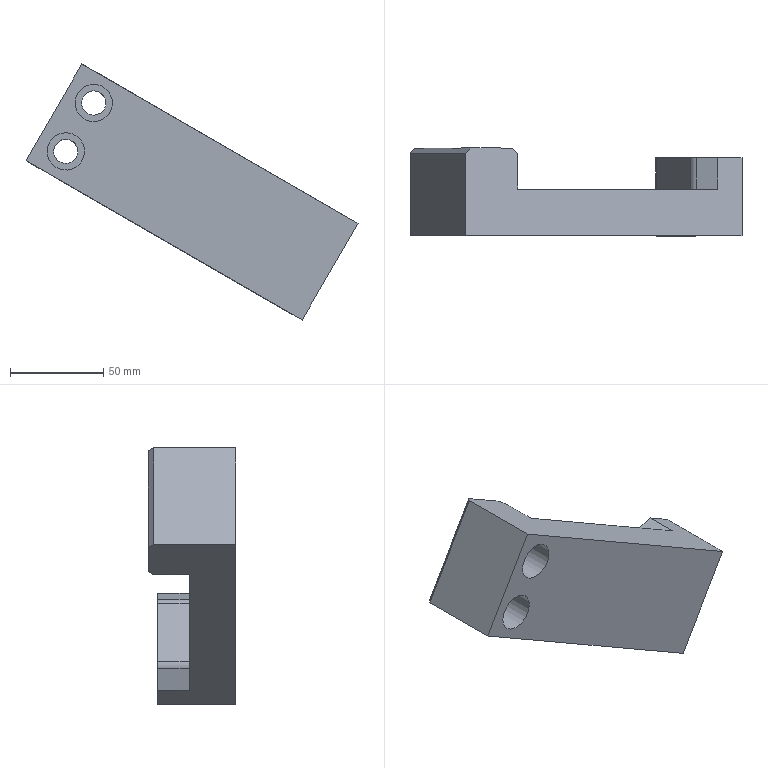Part | NX | features solid 2 | 1 solid | 22 faces | box 178.09 x 47 x 137.462 mm | volume 304062 mm3 | plane 16 | cylinder 6 | commonest cylinder face diameters 10 x2 13 x2 20 x2
STEP:
#1=CARTESIAN_POINT('',(239.,-415.,62.));
#2=VERTEX_POINT('',#1);
#3=CARTESIAN_POINT('',(239.,-371.,62.));
#4=VERTEX_POINT('',#3);
#5=CARTESIAN_POINT('',(239.,-415.,62.));
#6=DIRECTION('',(0.,1.,0.));
#7=VECTOR('',#6,1000.);
#8=LINE('',#5,#7);
#9=EDGE_CURVE('',#2,#4,#8,.T.);
#10=ORIENTED_EDGE('',*,*,#9,.F.);
#11=CARTESIAN_POINT('',(387.09,-415.,-23.5));
#12=VERTEX_POINT('',#11);
#13=CARTESIAN_POINT('',(387.09,-415.,-23.5));
#14=DIRECTION('',(-0.866,0.,0.5));
#15=VECTOR('',#14,1000.);
#16=LINE('',#13,#15);
#17=EDGE_CURVE('',#12,#2,#16,.T.);
#18=ORIENTED_EDGE('',*,*,#17,.F.);
#19=CARTESIAN_POINT('',(387.09,-373.,-23.5));
#20=VERTEX_POINT('',#19);
#21=CARTESIAN_POINT('',(387.09,-415.,-23.5));
#22=DIRECTION('',(0.,1.,0.));
#23=VECTOR('',#22,1000.);
#24=LINE('',#21,#23);
#25=EDGE_CURVE('',#12,#20,#24,.T.);
#26=ORIENTED_EDGE('',*,*,#25,.T.);
#27=CARTESIAN_POINT('',(374.1,-373.,-16.));
#28=VERTEX_POINT('',#27);
#29=CARTESIAN_POINT('',(387.09,-373.,-23.5));
#30=DIRECTION('',(-0.866,0.,0.5));
#31=VECTOR('',#30,1000.);
#32=LINE('',#29,#31);
#33=EDGE_CURVE('',#20,#28,#32,.T.);
#34=ORIENTED_EDGE('',*,*,#33,.T.);
#35=CARTESIAN_POINT('',(374.1,-390.,-16.));
#36=VERTEX_POINT('',#35);
#37=CARTESIAN_POINT('',(374.1,-415.,-16.));
#38=DIRECTION('',(0.,-1.,0.));
#39=VECTOR('',#38,1000.);
#40=LINE('',#37,#39);
#41=EDGE_CURVE('',#36,#28,#40,.F.);
#42=ORIENTED_EDGE('',*,*,#41,.F.);
#43=CARTESIAN_POINT('',(266.713,-390.,46.));
#44=VERTEX_POINT('',#43);
#45=CARTESIAN_POINT('',(387.09,-390.,-23.5));
#46=DIRECTION('',(-0.866,0.,0.5));
#47=VECTOR('',#46,1000.);
#48=LINE('',#45,#47);
#49=EDGE_CURVE('',#36,#44,#48,.T.);
#50=ORIENTED_EDGE('',*,*,#49,.T.);
#51=CARTESIAN_POINT('',(266.713,-371.,46.));
#52=VERTEX_POINT('',#51);
#53=CARTESIAN_POINT('',(266.713,-390.,46.));
#54=DIRECTION('',(0.,1.,0.));
#55=VECTOR('',#54,1000.);
#56=LINE('',#53,#55);
#57=EDGE_CURVE('',#44,#52,#56,.T.);
#58=ORIENTED_EDGE('',*,*,#57,.T.);
#59=CARTESIAN_POINT('',(264.115,-368.,47.5));
#60=VERTEX_POINT('',#59);
#61=CARTESIAN_POINT('',(345.954,-462.5,0.25));
#62=DIRECTION('',(-0.6124,0.7071,0.3536));
#63=VECTOR('',#62,1000.);
#64=LINE('',#61,#63);
#65=EDGE_CURVE('',#60,#52,#64,.F.);
#66=ORIENTED_EDGE('',*,*,#65,.F.);
#67=CARTESIAN_POINT('',(241.598,-368.,60.5));
#68=VERTEX_POINT('',#67);
#69=CARTESIAN_POINT('',(239.,-368.,62.));
#70=DIRECTION('',(0.866,0.,-0.5));
#71=VECTOR('',#70,1000.);
#72=LINE('',#69,#71);
#73=EDGE_CURVE('',#68,#60,#72,.T.);
#74=ORIENTED_EDGE('',*,*,#73,.F.);
#75=CARTESIAN_POINT('',(293.993,-307.5,30.25));
#76=DIRECTION('',(0.6124,0.7071,-0.3536));
#77=VECTOR('',#76,1000.);
#78=LINE('',#75,#77);
#79=EDGE_CURVE('',#4,#68,#78,.T.);
#80=ORIENTED_EDGE('',*,*,#79,.F.);
#81=EDGE_LOOP('',(#10,#18,#26,#34,#42,#50,#58,#66,#74,#80));
#82=FACE_BOUND('',#81,.T.);
#83=CARTESIAN_POINT('',(387.09,-415.,-23.5));
#84=DIRECTION('',(0.5,0.,0.866));
#85=DIRECTION('',(-0.866,0.,0.5));
#86=AXIS2_PLACEMENT_3D('',#83,#84,#85);
#87=PLANE('',#86);
#88=ADVANCED_FACE('',(#82),#87,.T.);
#89=CARTESIAN_POINT('',(359.404,-390.,-21.454));
#90=VERTEX_POINT('',#89);
#91=CARTESIAN_POINT('',(341.475,-390.,-52.508));
#92=VERTEX_POINT('',#91);
#93=CARTESIAN_POINT('',(365.44,-390.,-11.));
#94=DIRECTION('',(-0.5,0.,-0.866));
#95=VECTOR('',#94,1000.);
#96=LINE('',#93,#95);
#97=EDGE_CURVE('',#90,#92,#96,.T.);
#98=ORIENTED_EDGE('',*,*,#97,.F.);
#99=CARTESIAN_POINT('',(359.404,-373.,-21.454));
#100=VERTEX_POINT('',#99);
#101=CARTESIAN_POINT('',(359.404,-390.,-21.454));
#102=DIRECTION('',(0.,1.,0.));
#103=VECTOR('',#102,1000.);
#104=LINE('',#101,#103);
#105=EDGE_CURVE('',#100,#90,#104,.F.);
#106=ORIENTED_EDGE('',*,*,#105,.F.);
#107=CARTESIAN_POINT('',(341.475,-373.,-52.508));
#108=VERTEX_POINT('',#107);
#109=CARTESIAN_POINT('',(365.44,-373.,-11.));
#110=DIRECTION('',(-0.5,0.,-0.866));
#111=VECTOR('',#110,1000.);
#112=LINE('',#109,#111);
#113=EDGE_CURVE('',#100,#108,#112,.T.);
#114=ORIENTED_EDGE('',*,*,#113,.T.);
#115=CARTESIAN_POINT('',(341.475,-390.,-52.508));
#116=DIRECTION('',(0.,-1.,0.));
#117=VECTOR('',#116,1000.);
#118=LINE('',#115,#117);
#119=EDGE_CURVE('',#92,#108,#118,.F.);
#120=ORIENTED_EDGE('',*,*,#119,.F.);
#121=EDGE_LOOP('',(#98,#106,#114,#120));
#122=FACE_BOUND('',#121,.T.);
#123=CARTESIAN_POINT('',(365.44,-390.,-11.));
#124=DIRECTION('',(0.866,0.,-0.5));
#125=DIRECTION('',(-0.5,0.,-0.866));
#126=AXIS2_PLACEMENT_3D('',#123,#124,#125);
#127=PLANE('',#126);
#128=ADVANCED_FACE('',(#122),#127,.F.);
#129=ORIENTED_EDGE('',*,*,#113,.F.);
#130=CARTESIAN_POINT('',(362.44,-373.,-19.124));
#131=VERTEX_POINT('',#130);
#132=CARTESIAN_POINT('',(363.734,-373.,-23.954));
#133=DIRECTION('',(0.,1.,0.));
#134=DIRECTION('',(-0.5,0.,-0.866));
#135=AXIS2_PLACEMENT_3D('',#132,#133,#134);
#136=CIRCLE('',#135,5.);
#137=EDGE_CURVE('',#131,#100,#136,.F.);
#138=ORIENTED_EDGE('',*,*,#137,.F.);
#139=CARTESIAN_POINT('',(360.44,-373.,-19.66));
#140=DIRECTION('',(0.9659,0.,0.2588));
#141=VECTOR('',#140,1000.);
#142=LINE('',#139,#141);
#143=EDGE_CURVE('',#131,#28,#142,.T.);
#144=ORIENTED_EDGE('',*,*,#143,.T.);
#145=ORIENTED_EDGE('',*,*,#33,.F.);
#146=CARTESIAN_POINT('',(357.09,-373.,-75.462));
#147=VERTEX_POINT('',#146);
#148=CARTESIAN_POINT('',(387.09,-373.,-23.5));
#149=DIRECTION('',(-0.5,0.,-0.866));
#150=VECTOR('',#149,1000.);
#151=LINE('',#148,#150);
#152=EDGE_CURVE('',#20,#147,#151,.T.);
#153=ORIENTED_EDGE('',*,*,#152,.T.);
#154=CARTESIAN_POINT('',(344.1,-373.,-67.962));
#155=VERTEX_POINT('',#154);
#156=CARTESIAN_POINT('',(357.09,-373.,-75.462));
#157=DIRECTION('',(-0.866,0.,0.5));
#158=VECTOR('',#157,1000.);
#159=LINE('',#156,#158);
#160=EDGE_CURVE('',#147,#155,#159,.T.);
#161=ORIENTED_EDGE('',*,*,#160,.T.);
#162=CARTESIAN_POINT('',(340.976,-373.,-56.302));
#163=VERTEX_POINT('',#162);
#164=CARTESIAN_POINT('',(340.44,-373.,-54.301));
#165=DIRECTION('',(0.2588,0.,-0.9659));
#166=VECTOR('',#165,1000.);
#167=LINE('',#164,#166);
#168=EDGE_CURVE('',#163,#155,#167,.T.);
#169=ORIENTED_EDGE('',*,*,#168,.F.);
#170=CARTESIAN_POINT('',(345.805,-373.,-55.008));
#171=DIRECTION('',(0.,1.,0.));
#172=DIRECTION('',(-0.5,0.,-0.866));
#173=AXIS2_PLACEMENT_3D('',#170,#171,#172);
#174=CIRCLE('',#173,5.);
#175=EDGE_CURVE('',#108,#163,#174,.F.);
#176=ORIENTED_EDGE('',*,*,#175,.F.);
#177=EDGE_LOOP('',(#129,#138,#144,#145,#153,#161,#169,#176));
#178=FACE_BOUND('',#177,.T.);
#179=CARTESIAN_POINT('',(387.09,-373.,-23.5));
#180=DIRECTION('',(0.,-1.,0.));
#181=DIRECTION('',(-0.5,0.,-0.866));
#182=AXIS2_PLACEMENT_3D('',#179,#180,#181);
#183=PLANE('',#182);
#184=ADVANCED_FACE('',(#178),#183,.F.);
#185=ORIENTED_EDGE('',*,*,#49,.F.);
#186=CARTESIAN_POINT('',(362.44,-390.,-19.124));
#187=VERTEX_POINT('',#186);
#188=CARTESIAN_POINT('',(360.44,-390.,-19.66));
#189=DIRECTION('',(0.9659,0.,0.2588));
#190=VECTOR('',#189,1000.);
#191=LINE('',#188,#190);
#192=EDGE_CURVE('',#187,#36,#191,.T.);
#193=ORIENTED_EDGE('',*,*,#192,.F.);
#194=CARTESIAN_POINT('',(363.734,-390.,-23.954));
#195=DIRECTION('',(0.,1.,0.));
#196=DIRECTION('',(-0.866,0.,0.5));
#197=AXIS2_PLACEMENT_3D('',#194,#195,#196);
#198=CIRCLE('',#197,5.);
#199=EDGE_CURVE('',#90,#187,#198,.T.);
#200=ORIENTED_EDGE('',*,*,#199,.F.);
#201=ORIENTED_EDGE('',*,*,#97,.T.);
#202=CARTESIAN_POINT('',(340.976,-390.,-56.302));
#203=VERTEX_POINT('',#202);
#204=CARTESIAN_POINT('',(345.805,-390.,-55.008));
#205=DIRECTION('',(0.,1.,0.));
#206=DIRECTION('',(-0.866,0.,0.5));
#207=AXIS2_PLACEMENT_3D('',#204,#205,#206);
#208=CIRCLE('',#207,5.);
#209=EDGE_CURVE('',#203,#92,#208,.T.);
#210=ORIENTED_EDGE('',*,*,#209,.F.);
#211=CARTESIAN_POINT('',(344.1,-390.,-67.962));
#212=VERTEX_POINT('',#211);
#213=CARTESIAN_POINT('',(340.44,-390.,-54.301));
#214=DIRECTION('',(0.2588,0.,-0.9659));
#215=VECTOR('',#214,1000.);
#216=LINE('',#213,#215);
#217=EDGE_CURVE('',#203,#212,#216,.T.);
#218=ORIENTED_EDGE('',*,*,#217,.T.);
#219=CARTESIAN_POINT('',(236.713,-390.,-5.962));
#220=VERTEX_POINT('',#219);
#221=CARTESIAN_POINT('',(357.09,-390.,-75.462));
#222=DIRECTION('',(-0.866,0.,0.5));
#223=VECTOR('',#222,1000.);
#224=LINE('',#221,#223);
#225=EDGE_CURVE('',#212,#220,#224,.T.);
#226=ORIENTED_EDGE('',*,*,#225,.T.);
#227=CARTESIAN_POINT('',(266.713,-390.,46.));
#228=DIRECTION('',(-0.5,0.,-0.866));
#229=VECTOR('',#228,1000.);
#230=LINE('',#227,#229);
#231=EDGE_CURVE('',#44,#220,#230,.T.);
#232=ORIENTED_EDGE('',*,*,#231,.F.);
#233=EDGE_LOOP('',(#185,#193,#200,#201,#210,#218,#226,#232));
#234=FACE_BOUND('',#233,.T.);
#235=CARTESIAN_POINT('',(387.09,-390.,-23.5));
#236=DIRECTION('',(0.,-1.,0.));
#237=DIRECTION('',(-0.866,0.,0.5));
#238=AXIS2_PLACEMENT_3D('',#235,#236,#237);
#239=PLANE('',#238);
#240=ADVANCED_FACE('',(#234),#239,.F.);
#241=CARTESIAN_POINT('',(254.017,-415.,36.01));
#242=VERTEX_POINT('',#241);
#243=CARTESIAN_POINT('',(245.356,-415.,41.01));
#244=DIRECTION('',(0.,-1.,0.));
#245=DIRECTION('',(0.866,0.,-0.5));
#246=AXIS2_PLACEMENT_3D('',#243,#244,#245);
#247=CIRCLE('',#246,10.);
#248=EDGE_CURVE('',#242,#242,#247,.T.);
#249=ORIENTED_EDGE('',*,*,#248,.F.);
#250=EDGE_LOOP('',(#249));
#251=FACE_BOUND('',#250,.T.);
#252=CARTESIAN_POINT('',(239.017,-415.,10.029));
#253=VERTEX_POINT('',#252);
#254=CARTESIAN_POINT('',(230.356,-415.,15.029));
#255=DIRECTION('',(0.,-1.,0.));
#256=DIRECTION('',(0.866,0.,-0.5));
#257=AXIS2_PLACEMENT_3D('',#254,#255,#256);
#258=CIRCLE('',#257,10.);
#259=EDGE_CURVE('',#253,#253,#258,.T.);
#260=ORIENTED_EDGE('',*,*,#259,.F.);
#261=EDGE_LOOP('',(#260));
#262=FACE_BOUND('',#261,.T.);
#263=CARTESIAN_POINT('',(357.09,-415.,-75.462));
#264=VERTEX_POINT('',#263);
#265=CARTESIAN_POINT('',(387.09,-415.,-23.5));
#266=DIRECTION('',(0.5,0.,0.866));
#267=VECTOR('',#266,1000.);
#268=LINE('',#265,#267);
#269=EDGE_CURVE('',#12,#264,#268,.F.);
#270=ORIENTED_EDGE('',*,*,#269,.F.);
#271=ORIENTED_EDGE('',*,*,#17,.T.);
#272=CARTESIAN_POINT('',(209.,-415.,10.038));
#273=VERTEX_POINT('',#272);
#274=CARTESIAN_POINT('',(239.,-415.,62.));
#275=DIRECTION('',(0.5,0.,0.866));
#276=VECTOR('',#275,1000.);
#277=LINE('',#274,#276);
#278=EDGE_CURVE('',#2,#273,#277,.F.);
#279=ORIENTED_EDGE('',*,*,#278,.T.);
#280=CARTESIAN_POINT('',(357.09,-415.,-75.462));
#281=DIRECTION('',(-0.866,0.,0.5));
#282=VECTOR('',#281,1000.);
#283=LINE('',#280,#282);
#284=EDGE_CURVE('',#264,#273,#283,.T.);
#285=ORIENTED_EDGE('',*,*,#284,.F.);
#286=EDGE_LOOP('',(#270,#271,#279,#285));
#287=FACE_BOUND('',#286,.T.);
#288=CARTESIAN_POINT('',(387.09,-415.,-23.5));
#289=DIRECTION('',(0.,-1.,0.));
#290=DIRECTION('',(-0.866,0.,0.5));
#291=AXIS2_PLACEMENT_3D('',#288,#289,#290);
#292=PLANE('',#291);
#293=ADVANCED_FACE('',(#251,#262,#287),#292,.T.);
#294=CARTESIAN_POINT('',(209.,-371.,10.038));
#295=VERTEX_POINT('',#294);
#296=CARTESIAN_POINT('',(209.,-415.,10.038));
#297=DIRECTION('',(0.,1.,0.));
#298=VECTOR('',#297,1000.);
#299=LINE('',#296,#298);
#300=EDGE_CURVE('',#273,#295,#299,.T.);
#301=ORIENTED_EDGE('',*,*,#300,.F.);
#302=ORIENTED_EDGE('',*,*,#278,.F.);
#303=ORIENTED_EDGE('',*,*,#9,.T.);
#304=CARTESIAN_POINT('',(239.,-371.,62.));
#305=DIRECTION('',(-0.5,0.,-0.866));
#306=VECTOR('',#305,1000.);
#307=LINE('',#304,#306);
#308=EDGE_CURVE('',#295,#4,#307,.F.);
#309=ORIENTED_EDGE('',*,*,#308,.F.);
#310=EDGE_LOOP('',(#301,#302,#303,#309));
#311=FACE_BOUND('',#310,.T.);
#312=CARTESIAN_POINT('',(239.,-415.,62.));
#313=DIRECTION('',(-0.866,0.,0.5));
#314=DIRECTION('',(0.,1.,0.));
#315=AXIS2_PLACEMENT_3D('',#312,#313,#314);
#316=PLANE('',#315);
#317=ADVANCED_FACE('',(#311),#316,.T.);
#318=ORIENTED_EDGE('',*,*,#25,.F.);
#319=ORIENTED_EDGE('',*,*,#269,.T.);
#320=CARTESIAN_POINT('',(357.09,-415.,-75.462));
#321=DIRECTION('',(0.,1.,0.));
#322=VECTOR('',#321,1000.);
#323=LINE('',#320,#322);
#324=EDGE_CURVE('',#264,#147,#323,.T.);
#325=ORIENTED_EDGE('',*,*,#324,.T.);
#326=ORIENTED_EDGE('',*,*,#152,.F.);
#327=EDGE_LOOP('',(#318,#319,#325,#326));
#328=FACE_BOUND('',#327,.T.);
#329=CARTESIAN_POINT('',(387.09,-415.,-23.5));
#330=DIRECTION('',(-0.866,0.,0.5));
#331=DIRECTION('',(0.,1.,0.));
#332=AXIS2_PLACEMENT_3D('',#329,#330,#331);
#333=PLANE('',#332);
#334=ADVANCED_FACE('',(#328),#333,.F.);
#335=CARTESIAN_POINT('',(211.598,-368.,8.538));
#336=VERTEX_POINT('',#335);
#337=CARTESIAN_POINT('',(234.115,-368.,-4.462));
#338=VERTEX_POINT('',#337);
#339=CARTESIAN_POINT('',(357.09,-368.,-75.462));
#340=DIRECTION('',(-0.866,0.,0.5));
#341=VECTOR('',#340,1000.);
#342=LINE('',#339,#341);
#343=EDGE_CURVE('',#336,#338,#342,.F.);
#344=ORIENTED_EDGE('',*,*,#343,.T.);
#345=CARTESIAN_POINT('',(236.713,-371.,-5.962));
#346=VERTEX_POINT('',#345);
#347=CARTESIAN_POINT('',(236.713,-371.,-5.962));
#348=DIRECTION('',(0.6124,-0.7071,-0.3536));
#349=VECTOR('',#348,1000.);
#350=LINE('',#347,#349);
#351=EDGE_CURVE('',#346,#338,#350,.F.);
#352=ORIENTED_EDGE('',*,*,#351,.F.);
#353=CARTESIAN_POINT('',(236.713,-390.,-5.962));
#354=DIRECTION('',(0.,1.,0.));
#355=VECTOR('',#354,1000.);
#356=LINE('',#353,#355);
#357=EDGE_CURVE('',#220,#346,#356,.T.);
#358=ORIENTED_EDGE('',*,*,#357,.F.);
#359=ORIENTED_EDGE('',*,*,#225,.F.);
#360=CARTESIAN_POINT('',(344.1,-415.,-67.962));
#361=DIRECTION('',(0.,-1.,0.));
#362=VECTOR('',#361,1000.);
#363=LINE('',#360,#362);
#364=EDGE_CURVE('',#155,#212,#363,.T.);
#365=ORIENTED_EDGE('',*,*,#364,.F.);
#366=ORIENTED_EDGE('',*,*,#160,.F.);
#367=ORIENTED_EDGE('',*,*,#324,.F.);
#368=ORIENTED_EDGE('',*,*,#284,.T.);
#369=ORIENTED_EDGE('',*,*,#300,.T.);
#370=CARTESIAN_POINT('',(211.598,-368.,8.538));
#371=DIRECTION('',(-0.6124,-0.7071,0.3536));
#372=VECTOR('',#371,1000.);
#373=LINE('',#370,#372);
#374=EDGE_CURVE('',#336,#295,#373,.T.);
#375=ORIENTED_EDGE('',*,*,#374,.F.);
#376=EDGE_LOOP('',(#344,#352,#358,#359,#365,#366,#367,#368,#369,#375));
#377=FACE_BOUND('',#376,.T.);
#378=CARTESIAN_POINT('',(357.09,-415.,-75.462));
#379=DIRECTION('',(0.5,0.,0.866));
#380=DIRECTION('',(-0.866,0.,0.5));
#381=AXIS2_PLACEMENT_3D('',#378,#379,#380);
#382=PLANE('',#381);
#383=ADVANCED_FACE('',(#377),#382,.F.);
#384=ORIENTED_EDGE('',*,*,#57,.F.);
#385=ORIENTED_EDGE('',*,*,#231,.T.);
#386=ORIENTED_EDGE('',*,*,#357,.T.);
#387=CARTESIAN_POINT('',(266.713,-371.,46.));
#388=DIRECTION('',(0.5,0.,0.866));
#389=VECTOR('',#388,1000.);
#390=LINE('',#387,#389);
#391=EDGE_CURVE('',#52,#346,#390,.F.);
#392=ORIENTED_EDGE('',*,*,#391,.F.);
#393=EDGE_LOOP('',(#384,#385,#386,#392));
#394=FACE_BOUND('',#393,.T.);
#395=CARTESIAN_POINT('',(266.713,-390.,46.));
#396=DIRECTION('',(-0.866,0.,0.5));
#397=DIRECTION('',(-0.5,0.,-0.866));
#398=AXIS2_PLACEMENT_3D('',#395,#396,#397);
#399=PLANE('',#398);
#400=ADVANCED_FACE('',(#394),#399,.F.);
#401=CARTESIAN_POINT('',(242.106,-368.,35.38));
#402=VERTEX_POINT('',#401);
#403=CARTESIAN_POINT('',(245.356,-368.,41.01));
#404=DIRECTION('',(0.,1.,0.));
#405=DIRECTION('',(-0.5,0.,-0.866));
#406=AXIS2_PLACEMENT_3D('',#403,#404,#405);
#407=CIRCLE('',#406,6.5);
#408=EDGE_CURVE('',#402,#402,#407,.F.);
#409=ORIENTED_EDGE('',*,*,#408,.T.);
#410=EDGE_LOOP('',(#409));
#411=FACE_BOUND('',#410,.T.);
#412=CARTESIAN_POINT('',(227.106,-368.,9.4));
#413=VERTEX_POINT('',#412);
#414=CARTESIAN_POINT('',(230.356,-368.,15.029));
#415=DIRECTION('',(0.,1.,0.));
#416=DIRECTION('',(-0.5,0.,-0.866));
#417=AXIS2_PLACEMENT_3D('',#414,#415,#416);
#418=CIRCLE('',#417,6.5);
#419=EDGE_CURVE('',#413,#413,#418,.F.);
#420=ORIENTED_EDGE('',*,*,#419,.T.);
#421=EDGE_LOOP('',(#420));
#422=FACE_BOUND('',#421,.T.);
#423=ORIENTED_EDGE('',*,*,#73,.T.);
#424=CARTESIAN_POINT('',(264.115,-368.,47.5));
#425=DIRECTION('',(-0.5,0.,-0.866));
#426=VECTOR('',#425,1000.);
#427=LINE('',#424,#426);
#428=EDGE_CURVE('',#338,#60,#427,.F.);
#429=ORIENTED_EDGE('',*,*,#428,.F.);
#430=ORIENTED_EDGE('',*,*,#343,.F.);
#431=CARTESIAN_POINT('',(211.598,-368.,8.538));
#432=DIRECTION('',(0.5,0.,0.866));
#433=VECTOR('',#432,1000.);
#434=LINE('',#431,#433);
#435=EDGE_CURVE('',#68,#336,#434,.F.);
#436=ORIENTED_EDGE('',*,*,#435,.F.);
#437=EDGE_LOOP('',(#423,#429,#430,#436));
#438=FACE_BOUND('',#437,.T.);
#439=CARTESIAN_POINT('',(387.09,-368.,-23.5));
#440=DIRECTION('',(0.,-1.,0.));
#441=DIRECTION('',(-0.5,0.,-0.866));
#442=AXIS2_PLACEMENT_3D('',#439,#440,#441);
#443=PLANE('',#442);
#444=ADVANCED_FACE('',(#411,#422,#438),#443,.F.);
#445=ORIENTED_EDGE('',*,*,#168,.T.);
#446=ORIENTED_EDGE('',*,*,#364,.T.);
#447=ORIENTED_EDGE('',*,*,#217,.F.);
#448=CARTESIAN_POINT('',(340.976,-373.,-56.302));
#449=DIRECTION('',(0.,-1.,0.));
#450=VECTOR('',#449,1000.);
#451=LINE('',#448,#450);
#452=EDGE_CURVE('',#163,#203,#451,.T.);
#453=ORIENTED_EDGE('',*,*,#452,.F.);
#454=EDGE_LOOP('',(#445,#446,#447,#453));
#455=FACE_BOUND('',#454,.T.);
#456=CARTESIAN_POINT('',(340.44,-373.,-54.301));
#457=DIRECTION('',(0.9659,0.,0.2588));
#458=DIRECTION('',(0.2588,0.,-0.9659));
#459=AXIS2_PLACEMENT_3D('',#456,#457,#458);
#460=PLANE('',#459);
#461=ADVANCED_FACE('',(#455),#460,.F.);
#462=ORIENTED_EDGE('',*,*,#192,.T.);
#463=ORIENTED_EDGE('',*,*,#41,.T.);
#464=ORIENTED_EDGE('',*,*,#143,.F.);
#465=CARTESIAN_POINT('',(362.44,-373.,-19.124));
#466=DIRECTION('',(0.,-1.,0.));
#467=VECTOR('',#466,1000.);
#468=LINE('',#465,#467);
#469=EDGE_CURVE('',#187,#131,#468,.F.);
#470=ORIENTED_EDGE('',*,*,#469,.F.);
#471=EDGE_LOOP('',(#462,#463,#464,#470));
#472=FACE_BOUND('',#471,.T.);
#473=CARTESIAN_POINT('',(360.44,-373.,-19.66));
#474=DIRECTION('',(0.2588,0.,-0.9659));
#475=DIRECTION('',(0.9659,0.,0.2588));
#476=AXIS2_PLACEMENT_3D('',#473,#474,#475);
#477=PLANE('',#476);
#478=ADVANCED_FACE('',(#472),#477,.F.);
#479=ORIENTED_EDGE('',*,*,#175,.T.);
#480=ORIENTED_EDGE('',*,*,#452,.T.);
#481=ORIENTED_EDGE('',*,*,#209,.T.);
#482=ORIENTED_EDGE('',*,*,#119,.T.);
#483=EDGE_LOOP('',(#479,#480,#481,#482));
#484=FACE_BOUND('',#483,.T.);
#485=CARTESIAN_POINT('',(345.805,-373.,-55.008));
#486=DIRECTION('',(0.,-1.,0.));
#487=DIRECTION('',(-0.5,0.,-0.866));
#488=AXIS2_PLACEMENT_3D('',#485,#486,#487);
#489=CYLINDRICAL_SURFACE('',#488,5.);
#490=ADVANCED_FACE('',(#484),#489,.T.);
#491=ORIENTED_EDGE('',*,*,#137,.T.);
#492=ORIENTED_EDGE('',*,*,#105,.T.);
#493=ORIENTED_EDGE('',*,*,#199,.T.);
#494=ORIENTED_EDGE('',*,*,#469,.T.);
#495=EDGE_LOOP('',(#491,#492,#493,#494));
#496=FACE_BOUND('',#495,.T.);
#497=CARTESIAN_POINT('',(363.734,-390.,-23.954));
#498=DIRECTION('',(0.,-1.,0.));
#499=DIRECTION('',(-0.5,0.,-0.866));
#500=AXIS2_PLACEMENT_3D('',#497,#498,#499);
#501=CYLINDRICAL_SURFACE('',#500,5.);
#502=ADVANCED_FACE('',(#496),#501,.T.);
#503=ORIENTED_EDGE('',*,*,#419,.F.);
#504=EDGE_LOOP('',(#503));
#505=FACE_BOUND('',#504,.T.);
#506=CARTESIAN_POINT('',(235.986,-400.,11.779));
#507=VERTEX_POINT('',#506);
#508=CARTESIAN_POINT('',(230.356,-400.,15.029));
#509=DIRECTION('',(0.,-1.,0.));
#510=DIRECTION('',(0.866,0.,-0.5));
#511=AXIS2_PLACEMENT_3D('',#508,#509,#510);
#512=CIRCLE('',#511,6.5);
#513=EDGE_CURVE('',#507,#507,#512,.T.);
#514=ORIENTED_EDGE('',*,*,#513,.T.);
#515=EDGE_LOOP('',(#514));
#516=FACE_BOUND('',#515,.T.);
#517=CARTESIAN_POINT('',(230.356,-315.,15.029));
#518=DIRECTION('',(0.,1.,0.));
#519=DIRECTION('',(0.866,0.,-0.5));
#520=AXIS2_PLACEMENT_3D('',#517,#518,#519);
#521=CYLINDRICAL_SURFACE('',#520,6.5);
#522=ADVANCED_FACE('',(#505,#516),#521,.F.);
#523=ORIENTED_EDGE('',*,*,#513,.F.);
#524=EDGE_LOOP('',(#523));
#525=FACE_BOUND('',#524,.T.);
#526=CARTESIAN_POINT('',(239.017,-400.,10.029));
#527=VERTEX_POINT('',#526);
#528=CARTESIAN_POINT('',(230.356,-400.,15.029));
#529=DIRECTION('',(0.,-1.,0.));
#530=DIRECTION('',(0.866,0.,-0.5));
#531=AXIS2_PLACEMENT_3D('',#528,#529,#530);
#532=CIRCLE('',#531,10.);
#533=EDGE_CURVE('',#527,#527,#532,.T.);
#534=ORIENTED_EDGE('',*,*,#533,.T.);
#535=EDGE_LOOP('',(#534));
#536=FACE_BOUND('',#535,.T.);
#537=CARTESIAN_POINT('',(230.356,-400.,15.029));
#538=DIRECTION('',(0.,1.,0.));
#539=DIRECTION('',(0.866,0.,-0.5));
#540=AXIS2_PLACEMENT_3D('',#537,#538,#539);
#541=PLANE('',#540);
#542=ADVANCED_FACE('',(#525,#536),#541,.F.);
#543=ORIENTED_EDGE('',*,*,#533,.F.);
#544=EDGE_LOOP('',(#543));
#545=FACE_BOUND('',#544,.T.);
#546=ORIENTED_EDGE('',*,*,#259,.T.);
#547=EDGE_LOOP('',(#546));
#548=FACE_BOUND('',#547,.T.);
#549=CARTESIAN_POINT('',(230.356,-415.,15.029));
#550=DIRECTION('',(0.,1.,0.));
#551=DIRECTION('',(0.866,0.,-0.5));
#552=AXIS2_PLACEMENT_3D('',#549,#550,#551);
#553=CYLINDRICAL_SURFACE('',#552,10.);
#554=ADVANCED_FACE('',(#545,#548),#553,.F.);
#555=ORIENTED_EDGE('',*,*,#408,.F.);
#556=EDGE_LOOP('',(#555));
#557=FACE_BOUND('',#556,.T.);
#558=CARTESIAN_POINT('',(250.986,-400.,37.76));
#559=VERTEX_POINT('',#558);
#560=CARTESIAN_POINT('',(245.356,-400.,41.01));
#561=DIRECTION('',(0.,-1.,0.));
#562=DIRECTION('',(0.866,0.,-0.5));
#563=AXIS2_PLACEMENT_3D('',#560,#561,#562);
#564=CIRCLE('',#563,6.5);
#565=EDGE_CURVE('',#559,#559,#564,.T.);
#566=ORIENTED_EDGE('',*,*,#565,.T.);
#567=EDGE_LOOP('',(#566));
#568=FACE_BOUND('',#567,.T.);
#569=CARTESIAN_POINT('',(245.356,-315.,41.01));
#570=DIRECTION('',(0.,1.,0.));
#571=DIRECTION('',(0.866,0.,-0.5));
#572=AXIS2_PLACEMENT_3D('',#569,#570,#571);
#573=CYLINDRICAL_SURFACE('',#572,6.5);
#574=ADVANCED_FACE('',(#557,#568),#573,.F.);
#575=ORIENTED_EDGE('',*,*,#565,.F.);
#576=EDGE_LOOP('',(#575));
#577=FACE_BOUND('',#576,.T.);
#578=CARTESIAN_POINT('',(254.017,-400.,36.01));
#579=VERTEX_POINT('',#578);
#580=CARTESIAN_POINT('',(245.356,-400.,41.01));
#581=DIRECTION('',(0.,-1.,0.));
#582=DIRECTION('',(0.866,0.,-0.5));
#583=AXIS2_PLACEMENT_3D('',#580,#581,#582);
#584=CIRCLE('',#583,10.);
#585=EDGE_CURVE('',#579,#579,#584,.T.);
#586=ORIENTED_EDGE('',*,*,#585,.T.);
#587=EDGE_LOOP('',(#586));
#588=FACE_BOUND('',#587,.T.);
#589=CARTESIAN_POINT('',(245.356,-400.,41.01));
#590=DIRECTION('',(0.,1.,0.));
#591=DIRECTION('',(0.866,0.,-0.5));
#592=AXIS2_PLACEMENT_3D('',#589,#590,#591);
#593=PLANE('',#592);
#594=ADVANCED_FACE('',(#577,#588),#593,.F.);
#595=ORIENTED_EDGE('',*,*,#585,.F.);
#596=EDGE_LOOP('',(#595));
#597=FACE_BOUND('',#596,.T.);
#598=ORIENTED_EDGE('',*,*,#248,.T.);
#599=EDGE_LOOP('',(#598));
#600=FACE_BOUND('',#599,.T.);
#601=CARTESIAN_POINT('',(245.356,-415.,41.01));
#602=DIRECTION('',(0.,1.,0.));
#603=DIRECTION('',(0.866,0.,-0.5));
#604=AXIS2_PLACEMENT_3D('',#601,#602,#603);
#605=CYLINDRICAL_SURFACE('',#604,10.);
#606=ADVANCED_FACE('',(#597,#600),#605,.F.);
#607=ORIENTED_EDGE('',*,*,#79,.T.);
#608=ORIENTED_EDGE('',*,*,#435,.T.);
#609=ORIENTED_EDGE('',*,*,#374,.T.);
#610=ORIENTED_EDGE('',*,*,#308,.T.);
#611=EDGE_LOOP('',(#607,#608,#609,#610));
#612=FACE_BOUND('',#611,.T.);
#613=CARTESIAN_POINT('',(241.598,-368.,60.5));
#614=DIRECTION('',(-0.6124,0.7071,0.3536));
#615=DIRECTION('',(0.6124,0.7071,-0.3536));
#616=AXIS2_PLACEMENT_3D('',#613,#614,#615);
#617=PLANE('',#616);
#618=ADVANCED_FACE('',(#612),#617,.T.);
#619=ORIENTED_EDGE('',*,*,#65,.T.);
#620=ORIENTED_EDGE('',*,*,#391,.T.);
#621=ORIENTED_EDGE('',*,*,#351,.T.);
#622=ORIENTED_EDGE('',*,*,#428,.T.);
#623=EDGE_LOOP('',(#619,#620,#621,#622));
#624=FACE_BOUND('',#623,.T.);
#625=CARTESIAN_POINT('',(266.713,-371.,46.));
#626=DIRECTION('',(-0.6124,-0.7071,0.3536));
#627=DIRECTION('',(-0.6124,0.7071,0.3536));
#628=AXIS2_PLACEMENT_3D('',#625,#626,#627);
#629=PLANE('',#628);
#630=ADVANCED_FACE('',(#624),#629,.F.);
#631=CLOSED_SHELL('',(#88,#128,#184,#240,#293,#317,#334,#383,#400,#444,#461,#478,#490,#502,#522,#542,#554,#574,#594,#606,#618,#630));
#632=MANIFOLD_SOLID_BREP('',#631);
#633=(LENGTH_UNIT()NAMED_UNIT(*)SI_UNIT(.MILLI.,.METRE.));
#634=UNCERTAINTY_MEASURE_WITH_UNIT(LENGTH_MEASURE(0.00001),#633,'','');
#635=(NAMED_UNIT(*)PLANE_ANGLE_UNIT()SI_UNIT($,.RADIAN.));
#636=(NAMED_UNIT(*)SI_UNIT($,.STERADIAN.)SOLID_ANGLE_UNIT());
#637=(GEOMETRIC_REPRESENTATION_CONTEXT(3)GLOBAL_UNCERTAINTY_ASSIGNED_CONTEXT((#634))GLOBAL_UNIT_ASSIGNED_CONTEXT((#633,#635,#636))REPRESENTATION_CONTEXT('',''));
#638=ADVANCED_BREP_SHAPE_REPRESENTATION('',(#632),#637);